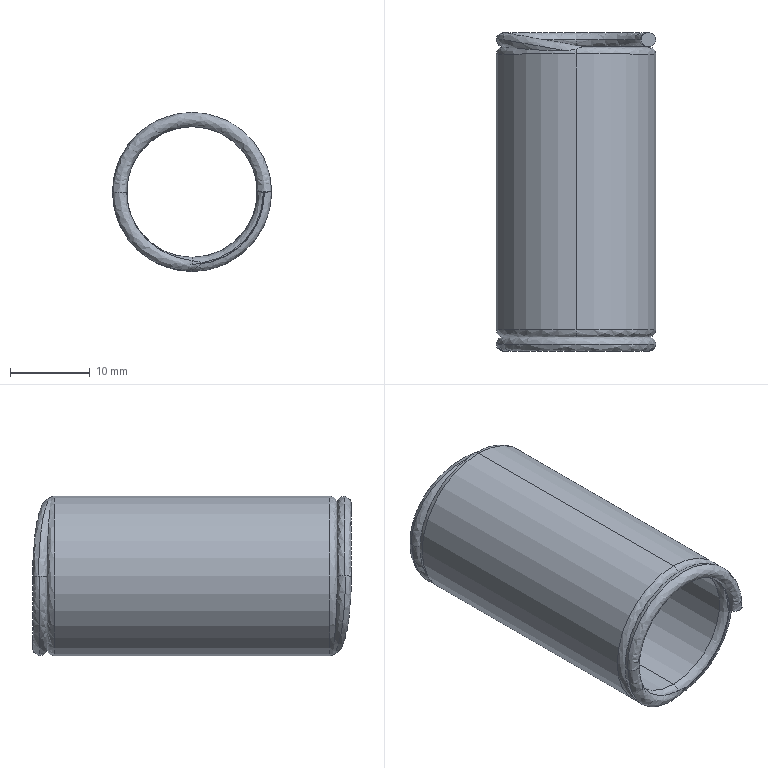Part | STEP file | UL20_40 round-wire coil spring_UL20-40 | 1 solid | 28 faces | box 20 x 40 x 20 mm | volume 3902 mm3 | spline 20 | cylinder 4 | plane 4 | commonest cylinder face diameters 16.4 x2 20 x2